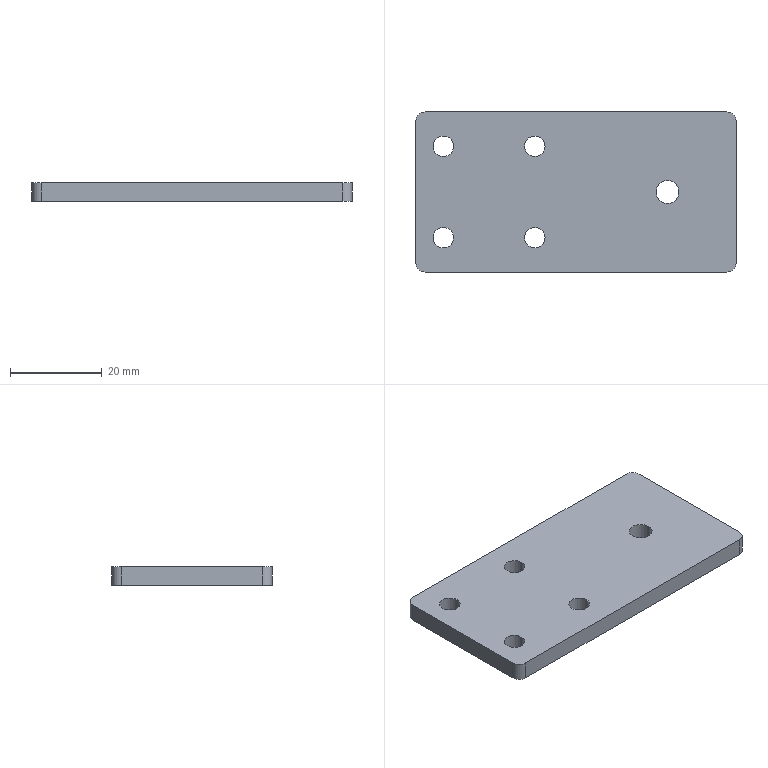Part | NX | features BREP 1 | 1 solid | 20 faces | box 70 x 35 x 4 mm | volume 9453 mm3 | cylinder 14 | plane 6 | commonest cylinder face diameters 4.5 x8 4 x4 5 x2
STEP:
#1=CARTESIAN_POINT('',(33.,-17.5,4.));
#2=VERTEX_POINT('',#1);
#3=CARTESIAN_POINT('',(35.,-15.5,4.));
#4=VERTEX_POINT('',#3);
#5=CARTESIAN_POINT('',(33.,-15.5,4.));
#6=DIRECTION('',(0.,0.,1.));
#7=DIRECTION('',(1.,0.,0.));
#8=AXIS2_PLACEMENT_3D('',#5,#6,#7);
#9=CIRCLE('',#8,2.);
#10=EDGE_CURVE('',#2,#4,#9,.T.);
#11=ORIENTED_EDGE('',*,*,#10,.F.);
#12=CARTESIAN_POINT('',(33.,-17.5,0.));
#13=VERTEX_POINT('',#12);
#14=CARTESIAN_POINT('',(33.,-17.5,4.));
#15=DIRECTION('',(0.,0.,1.));
#16=VECTOR('',#15,1000.);
#17=LINE('',#14,#16);
#18=EDGE_CURVE('',#13,#2,#17,.T.);
#19=ORIENTED_EDGE('',*,*,#18,.F.);
#20=CARTESIAN_POINT('',(35.,-15.5,0.));
#21=VERTEX_POINT('',#20);
#22=CARTESIAN_POINT('',(33.,-15.5,0.));
#23=DIRECTION('',(0.,0.,-1.));
#24=DIRECTION('',(1.,0.,0.));
#25=AXIS2_PLACEMENT_3D('',#22,#23,#24);
#26=CIRCLE('',#25,2.);
#27=EDGE_CURVE('',#21,#13,#26,.T.);
#28=ORIENTED_EDGE('',*,*,#27,.F.);
#29=CARTESIAN_POINT('',(35.,-15.5,4.));
#30=DIRECTION('',(0.,0.,-1.));
#31=VECTOR('',#30,1000.);
#32=LINE('',#29,#31);
#33=EDGE_CURVE('',#4,#21,#32,.T.);
#34=ORIENTED_EDGE('',*,*,#33,.F.);
#35=EDGE_LOOP('',(#11,#19,#28,#34));
#36=FACE_BOUND('',#35,.T.);
#37=CARTESIAN_POINT('',(33.,-15.5,4.));
#38=DIRECTION('',(0.,0.,-1.));
#39=DIRECTION('',(-1.,0.,0.));
#40=AXIS2_PLACEMENT_3D('',#37,#38,#39);
#41=CYLINDRICAL_SURFACE('',#40,2.);
#42=ADVANCED_FACE('',(#36),#41,.T.);
#43=CARTESIAN_POINT('',(35.,15.5,4.));
#44=VERTEX_POINT('',#43);
#45=CARTESIAN_POINT('',(33.,17.5,4.));
#46=VERTEX_POINT('',#45);
#47=CARTESIAN_POINT('',(33.,15.5,4.));
#48=DIRECTION('',(0.,0.,1.));
#49=DIRECTION('',(1.,0.,0.));
#50=AXIS2_PLACEMENT_3D('',#47,#48,#49);
#51=CIRCLE('',#50,2.);
#52=EDGE_CURVE('',#44,#46,#51,.T.);
#53=ORIENTED_EDGE('',*,*,#52,.F.);
#54=CARTESIAN_POINT('',(35.,15.5,0.));
#55=VERTEX_POINT('',#54);
#56=CARTESIAN_POINT('',(35.,15.5,4.));
#57=DIRECTION('',(0.,0.,1.));
#58=VECTOR('',#57,1000.);
#59=LINE('',#56,#58);
#60=EDGE_CURVE('',#55,#44,#59,.T.);
#61=ORIENTED_EDGE('',*,*,#60,.F.);
#62=CARTESIAN_POINT('',(33.,17.5,0.));
#63=VERTEX_POINT('',#62);
#64=CARTESIAN_POINT('',(33.,15.5,0.));
#65=DIRECTION('',(0.,0.,-1.));
#66=DIRECTION('',(1.,0.,0.));
#67=AXIS2_PLACEMENT_3D('',#64,#65,#66);
#68=CIRCLE('',#67,2.);
#69=EDGE_CURVE('',#63,#55,#68,.T.);
#70=ORIENTED_EDGE('',*,*,#69,.F.);
#71=CARTESIAN_POINT('',(33.,17.5,4.));
#72=DIRECTION('',(0.,0.,-1.));
#73=VECTOR('',#72,1000.);
#74=LINE('',#71,#73);
#75=EDGE_CURVE('',#46,#63,#74,.T.);
#76=ORIENTED_EDGE('',*,*,#75,.F.);
#77=EDGE_LOOP('',(#53,#61,#70,#76));
#78=FACE_BOUND('',#77,.T.);
#79=CARTESIAN_POINT('',(33.,15.5,4.));
#80=DIRECTION('',(0.,0.,-1.));
#81=DIRECTION('',(-1.,0.,0.));
#82=AXIS2_PLACEMENT_3D('',#79,#80,#81);
#83=CYLINDRICAL_SURFACE('',#82,2.);
#84=ADVANCED_FACE('',(#78),#83,.T.);
#85=CARTESIAN_POINT('',(-35.,-15.5,4.));
#86=VERTEX_POINT('',#85);
#87=CARTESIAN_POINT('',(-33.,-17.5,4.));
#88=VERTEX_POINT('',#87);
#89=CARTESIAN_POINT('',(-33.,-15.5,4.));
#90=DIRECTION('',(0.,0.,1.));
#91=DIRECTION('',(1.,0.,0.));
#92=AXIS2_PLACEMENT_3D('',#89,#90,#91);
#93=CIRCLE('',#92,2.);
#94=EDGE_CURVE('',#86,#88,#93,.T.);
#95=ORIENTED_EDGE('',*,*,#94,.F.);
#96=CARTESIAN_POINT('',(-35.,-15.5,0.));
#97=VERTEX_POINT('',#96);
#98=CARTESIAN_POINT('',(-35.,-15.5,4.));
#99=DIRECTION('',(0.,0.,1.));
#100=VECTOR('',#99,1000.);
#101=LINE('',#98,#100);
#102=EDGE_CURVE('',#97,#86,#101,.T.);
#103=ORIENTED_EDGE('',*,*,#102,.F.);
#104=CARTESIAN_POINT('',(-33.,-17.5,0.));
#105=VERTEX_POINT('',#104);
#106=CARTESIAN_POINT('',(-33.,-15.5,0.));
#107=DIRECTION('',(0.,0.,-1.));
#108=DIRECTION('',(1.,0.,0.));
#109=AXIS2_PLACEMENT_3D('',#106,#107,#108);
#110=CIRCLE('',#109,2.);
#111=EDGE_CURVE('',#105,#97,#110,.T.);
#112=ORIENTED_EDGE('',*,*,#111,.F.);
#113=CARTESIAN_POINT('',(-33.,-17.5,4.));
#114=DIRECTION('',(0.,0.,-1.));
#115=VECTOR('',#114,1000.);
#116=LINE('',#113,#115);
#117=EDGE_CURVE('',#88,#105,#116,.T.);
#118=ORIENTED_EDGE('',*,*,#117,.F.);
#119=EDGE_LOOP('',(#95,#103,#112,#118));
#120=FACE_BOUND('',#119,.T.);
#121=CARTESIAN_POINT('',(-33.,-15.5,4.));
#122=DIRECTION('',(0.,0.,-1.));
#123=DIRECTION('',(-1.,0.,0.));
#124=AXIS2_PLACEMENT_3D('',#121,#122,#123);
#125=CYLINDRICAL_SURFACE('',#124,2.);
#126=ADVANCED_FACE('',(#120),#125,.T.);
#127=CARTESIAN_POINT('',(-33.,17.5,4.));
#128=VERTEX_POINT('',#127);
#129=CARTESIAN_POINT('',(-35.,15.5,4.));
#130=VERTEX_POINT('',#129);
#131=CARTESIAN_POINT('',(-33.,15.5,4.));
#132=DIRECTION('',(0.,0.,1.));
#133=DIRECTION('',(1.,0.,0.));
#134=AXIS2_PLACEMENT_3D('',#131,#132,#133);
#135=CIRCLE('',#134,2.);
#136=EDGE_CURVE('',#128,#130,#135,.T.);
#137=ORIENTED_EDGE('',*,*,#136,.F.);
#138=CARTESIAN_POINT('',(-33.,17.5,0.));
#139=VERTEX_POINT('',#138);
#140=CARTESIAN_POINT('',(-33.,17.5,4.));
#141=DIRECTION('',(0.,0.,1.));
#142=VECTOR('',#141,1000.);
#143=LINE('',#140,#142);
#144=EDGE_CURVE('',#139,#128,#143,.T.);
#145=ORIENTED_EDGE('',*,*,#144,.F.);
#146=CARTESIAN_POINT('',(-35.,15.5,0.));
#147=VERTEX_POINT('',#146);
#148=CARTESIAN_POINT('',(-33.,15.5,0.));
#149=DIRECTION('',(0.,0.,-1.));
#150=DIRECTION('',(1.,0.,0.));
#151=AXIS2_PLACEMENT_3D('',#148,#149,#150);
#152=CIRCLE('',#151,2.);
#153=EDGE_CURVE('',#147,#139,#152,.T.);
#154=ORIENTED_EDGE('',*,*,#153,.F.);
#155=CARTESIAN_POINT('',(-35.,15.5,4.));
#156=DIRECTION('',(0.,0.,-1.));
#157=VECTOR('',#156,1000.);
#158=LINE('',#155,#157);
#159=EDGE_CURVE('',#130,#147,#158,.T.);
#160=ORIENTED_EDGE('',*,*,#159,.F.);
#161=EDGE_LOOP('',(#137,#145,#154,#160));
#162=FACE_BOUND('',#161,.T.);
#163=CARTESIAN_POINT('',(-33.,15.5,4.));
#164=DIRECTION('',(0.,0.,-1.));
#165=DIRECTION('',(-1.,0.,0.));
#166=AXIS2_PLACEMENT_3D('',#163,#164,#165);
#167=CYLINDRICAL_SURFACE('',#166,2.);
#168=ADVANCED_FACE('',(#162),#167,.T.);
#169=CARTESIAN_POINT('',(-6.75,10.,4.));
#170=VERTEX_POINT('',#169);
#171=CARTESIAN_POINT('',(-6.75,10.,0.));
#172=VERTEX_POINT('',#171);
#173=CARTESIAN_POINT('',(-6.75,10.,0.));
#174=DIRECTION('',(0.,0.,-1.));
#175=VECTOR('',#174,1000.);
#176=LINE('',#173,#175);
#177=EDGE_CURVE('',#170,#172,#176,.T.);
#178=ORIENTED_EDGE('',*,*,#177,.F.);
#179=CARTESIAN_POINT('',(-11.25,10.,4.));
#180=VERTEX_POINT('',#179);
#181=CARTESIAN_POINT('',(-9.,10.,4.));
#182=DIRECTION('',(0.,0.,1.));
#183=DIRECTION('',(1.,0.,0.));
#184=AXIS2_PLACEMENT_3D('',#181,#182,#183);
#185=CIRCLE('',#184,2.25);
#186=EDGE_CURVE('',#170,#180,#185,.T.);
#187=ORIENTED_EDGE('',*,*,#186,.T.);
#188=CARTESIAN_POINT('',(-11.25,10.,0.));
#189=VERTEX_POINT('',#188);
#190=CARTESIAN_POINT('',(-11.25,10.,0.));
#191=DIRECTION('',(0.,0.,-1.));
#192=VECTOR('',#191,1000.);
#193=LINE('',#190,#192);
#194=EDGE_CURVE('',#180,#189,#193,.T.);
#195=ORIENTED_EDGE('',*,*,#194,.T.);
#196=CARTESIAN_POINT('',(-9.,10.,0.));
#197=DIRECTION('',(0.,0.,-1.));
#198=DIRECTION('',(-1.,0.,0.));
#199=AXIS2_PLACEMENT_3D('',#196,#197,#198);
#200=CIRCLE('',#199,2.25);
#201=EDGE_CURVE('',#189,#172,#200,.T.);
#202=ORIENTED_EDGE('',*,*,#201,.T.);
#203=EDGE_LOOP('',(#178,#187,#195,#202));
#204=FACE_BOUND('',#203,.T.);
#205=CARTESIAN_POINT('',(-9.,10.,0.));
#206=DIRECTION('',(0.,0.,-1.));
#207=DIRECTION('',(-1.,0.,0.));
#208=AXIS2_PLACEMENT_3D('',#205,#206,#207);
#209=CYLINDRICAL_SURFACE('',#208,2.25);
#210=ADVANCED_FACE('',(#204),#209,.F.);
#211=CARTESIAN_POINT('',(-26.75,-10.,4.));
#212=VERTEX_POINT('',#211);
#213=CARTESIAN_POINT('',(-26.75,-10.,0.));
#214=VERTEX_POINT('',#213);
#215=CARTESIAN_POINT('',(-26.75,-10.,0.));
#216=DIRECTION('',(0.,0.,-1.));
#217=VECTOR('',#216,1000.);
#218=LINE('',#215,#217);
#219=EDGE_CURVE('',#212,#214,#218,.T.);
#220=ORIENTED_EDGE('',*,*,#219,.F.);
#221=CARTESIAN_POINT('',(-31.25,-10.,4.));
#222=VERTEX_POINT('',#221);
#223=CARTESIAN_POINT('',(-29.,-10.,4.));
#224=DIRECTION('',(0.,0.,1.));
#225=DIRECTION('',(1.,0.,0.));
#226=AXIS2_PLACEMENT_3D('',#223,#224,#225);
#227=CIRCLE('',#226,2.25);
#228=EDGE_CURVE('',#212,#222,#227,.T.);
#229=ORIENTED_EDGE('',*,*,#228,.T.);
#230=CARTESIAN_POINT('',(-31.25,-10.,0.));
#231=VERTEX_POINT('',#230);
#232=CARTESIAN_POINT('',(-31.25,-10.,0.));
#233=DIRECTION('',(0.,0.,-1.));
#234=VECTOR('',#233,1000.);
#235=LINE('',#232,#234);
#236=EDGE_CURVE('',#222,#231,#235,.T.);
#237=ORIENTED_EDGE('',*,*,#236,.T.);
#238=CARTESIAN_POINT('',(-29.,-10.,0.));
#239=DIRECTION('',(0.,0.,-1.));
#240=DIRECTION('',(-1.,0.,0.));
#241=AXIS2_PLACEMENT_3D('',#238,#239,#240);
#242=CIRCLE('',#241,2.25);
#243=EDGE_CURVE('',#231,#214,#242,.T.);
#244=ORIENTED_EDGE('',*,*,#243,.T.);
#245=EDGE_LOOP('',(#220,#229,#237,#244));
#246=FACE_BOUND('',#245,.T.);
#247=CARTESIAN_POINT('',(-29.,-10.,0.));
#248=DIRECTION('',(0.,0.,-1.));
#249=DIRECTION('',(-1.,0.,0.));
#250=AXIS2_PLACEMENT_3D('',#247,#248,#249);
#251=CYLINDRICAL_SURFACE('',#250,2.25);
#252=ADVANCED_FACE('',(#246),#251,.F.);
#253=CARTESIAN_POINT('',(-6.75,-10.,4.));
#254=VERTEX_POINT('',#253);
#255=CARTESIAN_POINT('',(-6.75,-10.,0.));
#256=VERTEX_POINT('',#255);
#257=CARTESIAN_POINT('',(-6.75,-10.,0.));
#258=DIRECTION('',(0.,0.,-1.));
#259=VECTOR('',#258,1000.);
#260=LINE('',#257,#259);
#261=EDGE_CURVE('',#254,#256,#260,.T.);
#262=ORIENTED_EDGE('',*,*,#261,.F.);
#263=CARTESIAN_POINT('',(-11.25,-10.,4.));
#264=VERTEX_POINT('',#263);
#265=CARTESIAN_POINT('',(-9.,-10.,4.));
#266=DIRECTION('',(0.,0.,1.));
#267=DIRECTION('',(1.,0.,0.));
#268=AXIS2_PLACEMENT_3D('',#265,#266,#267);
#269=CIRCLE('',#268,2.25);
#270=EDGE_CURVE('',#254,#264,#269,.T.);
#271=ORIENTED_EDGE('',*,*,#270,.T.);
#272=CARTESIAN_POINT('',(-11.25,-10.,0.));
#273=VERTEX_POINT('',#272);
#274=CARTESIAN_POINT('',(-11.25,-10.,0.));
#275=DIRECTION('',(0.,0.,-1.));
#276=VECTOR('',#275,1000.);
#277=LINE('',#274,#276);
#278=EDGE_CURVE('',#264,#273,#277,.T.);
#279=ORIENTED_EDGE('',*,*,#278,.T.);
#280=CARTESIAN_POINT('',(-9.,-10.,0.));
#281=DIRECTION('',(0.,0.,-1.));
#282=DIRECTION('',(-1.,0.,0.));
#283=AXIS2_PLACEMENT_3D('',#280,#281,#282);
#284=CIRCLE('',#283,2.25);
#285=EDGE_CURVE('',#273,#256,#284,.T.);
#286=ORIENTED_EDGE('',*,*,#285,.T.);
#287=EDGE_LOOP('',(#262,#271,#279,#286));
#288=FACE_BOUND('',#287,.T.);
#289=CARTESIAN_POINT('',(-9.,-10.,0.));
#290=DIRECTION('',(0.,0.,-1.));
#291=DIRECTION('',(-1.,0.,0.));
#292=AXIS2_PLACEMENT_3D('',#289,#290,#291);
#293=CYLINDRICAL_SURFACE('',#292,2.25);
#294=ADVANCED_FACE('',(#288),#293,.F.);
#295=CARTESIAN_POINT('',(-26.75,10.,4.));
#296=VERTEX_POINT('',#295);
#297=CARTESIAN_POINT('',(-26.75,10.,0.));
#298=VERTEX_POINT('',#297);
#299=CARTESIAN_POINT('',(-26.75,10.,0.));
#300=DIRECTION('',(0.,0.,-1.));
#301=VECTOR('',#300,1000.);
#302=LINE('',#299,#301);
#303=EDGE_CURVE('',#296,#298,#302,.T.);
#304=ORIENTED_EDGE('',*,*,#303,.F.);
#305=CARTESIAN_POINT('',(-31.25,10.,4.));
#306=VERTEX_POINT('',#305);
#307=CARTESIAN_POINT('',(-29.,10.,4.));
#308=DIRECTION('',(0.,0.,1.));
#309=DIRECTION('',(1.,0.,0.));
#310=AXIS2_PLACEMENT_3D('',#307,#308,#309);
#311=CIRCLE('',#310,2.25);
#312=EDGE_CURVE('',#296,#306,#311,.T.);
#313=ORIENTED_EDGE('',*,*,#312,.T.);
#314=CARTESIAN_POINT('',(-31.25,10.,0.));
#315=VERTEX_POINT('',#314);
#316=CARTESIAN_POINT('',(-31.25,10.,0.));
#317=DIRECTION('',(0.,0.,-1.));
#318=VECTOR('',#317,1000.);
#319=LINE('',#316,#318);
#320=EDGE_CURVE('',#306,#315,#319,.T.);
#321=ORIENTED_EDGE('',*,*,#320,.T.);
#322=CARTESIAN_POINT('',(-29.,10.,0.));
#323=DIRECTION('',(0.,0.,-1.));
#324=DIRECTION('',(-1.,0.,0.));
#325=AXIS2_PLACEMENT_3D('',#322,#323,#324);
#326=CIRCLE('',#325,2.25);
#327=EDGE_CURVE('',#315,#298,#326,.T.);
#328=ORIENTED_EDGE('',*,*,#327,.T.);
#329=EDGE_LOOP('',(#304,#313,#321,#328));
#330=FACE_BOUND('',#329,.T.);
#331=CARTESIAN_POINT('',(-29.,10.,0.));
#332=DIRECTION('',(0.,0.,-1.));
#333=DIRECTION('',(-1.,0.,0.));
#334=AXIS2_PLACEMENT_3D('',#331,#332,#333);
#335=CYLINDRICAL_SURFACE('',#334,2.25);
#336=ADVANCED_FACE('',(#330),#335,.F.);
#337=CARTESIAN_POINT('',(17.5,0.,4.));
#338=VERTEX_POINT('',#337);
#339=CARTESIAN_POINT('',(17.5,0.,0.));
#340=VERTEX_POINT('',#339);
#341=CARTESIAN_POINT('',(17.5,0.,4.));
#342=DIRECTION('',(0.,0.,1.));
#343=VECTOR('',#342,1000.);
#344=LINE('',#341,#343);
#345=EDGE_CURVE('',#338,#340,#344,.F.);
#346=ORIENTED_EDGE('',*,*,#345,.T.);
#347=CARTESIAN_POINT('',(22.5,0.,0.));
#348=VERTEX_POINT('',#347);
#349=CARTESIAN_POINT('',(20.,0.,0.));
#350=DIRECTION('',(0.,0.,1.));
#351=DIRECTION('',(1.,0.,0.));
#352=AXIS2_PLACEMENT_3D('',#349,#350,#351);
#353=CIRCLE('',#352,2.5);
#354=EDGE_CURVE('',#348,#340,#353,.T.);
#355=ORIENTED_EDGE('',*,*,#354,.F.);
#356=CARTESIAN_POINT('',(22.5,0.,4.));
#357=VERTEX_POINT('',#356);
#358=CARTESIAN_POINT('',(22.5,0.,4.));
#359=DIRECTION('',(0.,0.,1.));
#360=VECTOR('',#359,1000.);
#361=LINE('',#358,#360);
#362=EDGE_CURVE('',#357,#348,#361,.F.);
#363=ORIENTED_EDGE('',*,*,#362,.F.);
#364=CARTESIAN_POINT('',(20.,0.,4.));
#365=DIRECTION('',(0.,0.,1.));
#366=DIRECTION('',(1.,0.,0.));
#367=AXIS2_PLACEMENT_3D('',#364,#365,#366);
#368=CIRCLE('',#367,2.5);
#369=EDGE_CURVE('',#357,#338,#368,.T.);
#370=ORIENTED_EDGE('',*,*,#369,.T.);
#371=EDGE_LOOP('',(#346,#355,#363,#370));
#372=FACE_BOUND('',#371,.T.);
#373=CARTESIAN_POINT('',(20.,0.,4.));
#374=DIRECTION('',(0.,0.,1.));
#375=DIRECTION('',(1.,0.,0.));
#376=AXIS2_PLACEMENT_3D('',#373,#374,#375);
#377=CYLINDRICAL_SURFACE('',#376,2.5);
#378=ADVANCED_FACE('',(#372),#377,.F.);
#379=CARTESIAN_POINT('',(-35.,17.5,0.));
#380=DIRECTION('',(0.,-1.,0.));
#381=VECTOR('',#380,1000.);
#382=LINE('',#379,#381);
#383=EDGE_CURVE('',#147,#97,#382,.T.);
#384=ORIENTED_EDGE('',*,*,#383,.F.);
#385=ORIENTED_EDGE('',*,*,#153,.T.);
#386=CARTESIAN_POINT('',(-35.,17.5,0.));
#387=DIRECTION('',(-1.,0.,0.));
#388=VECTOR('',#387,1000.);
#389=LINE('',#386,#388);
#390=EDGE_CURVE('',#63,#139,#389,.T.);
#391=ORIENTED_EDGE('',*,*,#390,.F.);
#392=ORIENTED_EDGE('',*,*,#69,.T.);
#393=CARTESIAN_POINT('',(35.,17.5,0.));
#394=DIRECTION('',(0.,1.,0.));
#395=VECTOR('',#394,1000.);
#396=LINE('',#393,#395);
#397=EDGE_CURVE('',#21,#55,#396,.T.);
#398=ORIENTED_EDGE('',*,*,#397,.F.);
#399=ORIENTED_EDGE('',*,*,#27,.T.);
#400=CARTESIAN_POINT('',(-35.,-17.5,0.));
#401=DIRECTION('',(1.,0.,0.));
#402=VECTOR('',#401,1000.);
#403=LINE('',#400,#402);
#404=EDGE_CURVE('',#105,#13,#403,.T.);
#405=ORIENTED_EDGE('',*,*,#404,.F.);
#406=ORIENTED_EDGE('',*,*,#111,.T.);
#407=EDGE_LOOP('',(#384,#385,#391,#392,#398,#399,#405,#406));
#408=FACE_BOUND('',#407,.T.);
#409=ORIENTED_EDGE('',*,*,#354,.T.);
#410=CARTESIAN_POINT('',(20.,0.,0.));
#411=DIRECTION('',(0.,0.,1.));
#412=DIRECTION('',(1.,0.,0.));
#413=AXIS2_PLACEMENT_3D('',#410,#411,#412);
#414=CIRCLE('',#413,2.5);
#415=EDGE_CURVE('',#340,#348,#414,.T.);
#416=ORIENTED_EDGE('',*,*,#415,.T.);
#417=EDGE_LOOP('',(#409,#416));
#418=FACE_BOUND('',#417,.T.);
#419=ORIENTED_EDGE('',*,*,#327,.F.);
#420=CARTESIAN_POINT('',(-29.,10.,0.));
#421=DIRECTION('',(0.,0.,-1.));
#422=DIRECTION('',(-1.,0.,0.));
#423=AXIS2_PLACEMENT_3D('',#420,#421,#422);
#424=CIRCLE('',#423,2.25);
#425=EDGE_CURVE('',#298,#315,#424,.T.);
#426=ORIENTED_EDGE('',*,*,#425,.F.);
#427=EDGE_LOOP('',(#419,#426));
#428=FACE_BOUND('',#427,.T.);
#429=ORIENTED_EDGE('',*,*,#285,.F.);
#430=CARTESIAN_POINT('',(-9.,-10.,0.));
#431=DIRECTION('',(0.,0.,-1.));
#432=DIRECTION('',(-1.,0.,0.));
#433=AXIS2_PLACEMENT_3D('',#430,#431,#432);
#434=CIRCLE('',#433,2.25);
#435=EDGE_CURVE('',#256,#273,#434,.T.);
#436=ORIENTED_EDGE('',*,*,#435,.F.);
#437=EDGE_LOOP('',(#429,#436));
#438=FACE_BOUND('',#437,.T.);
#439=ORIENTED_EDGE('',*,*,#243,.F.);
#440=CARTESIAN_POINT('',(-29.,-10.,0.));
#441=DIRECTION('',(0.,0.,-1.));
#442=DIRECTION('',(-1.,0.,0.));
#443=AXIS2_PLACEMENT_3D('',#440,#441,#442);
#444=CIRCLE('',#443,2.25);
#445=EDGE_CURVE('',#214,#231,#444,.T.);
#446=ORIENTED_EDGE('',*,*,#445,.F.);
#447=EDGE_LOOP('',(#439,#446));
#448=FACE_BOUND('',#447,.T.);
#449=ORIENTED_EDGE('',*,*,#201,.F.);
#450=CARTESIAN_POINT('',(-9.,10.,0.));
#451=DIRECTION('',(0.,0.,-1.));
#452=DIRECTION('',(-1.,0.,0.));
#453=AXIS2_PLACEMENT_3D('',#450,#451,#452);
#454=CIRCLE('',#453,2.25);
#455=EDGE_CURVE('',#172,#189,#454,.T.);
#456=ORIENTED_EDGE('',*,*,#455,.F.);
#457=EDGE_LOOP('',(#449,#456));
#458=FACE_BOUND('',#457,.T.);
#459=CARTESIAN_POINT('',(0.,0.,0.));
#460=DIRECTION('',(0.,0.,1.));
#461=DIRECTION('',(1.,0.,0.));
#462=AXIS2_PLACEMENT_3D('',#459,#460,#461);
#463=PLANE('',#462);
#464=ADVANCED_FACE('',(#408,#418,#428,#438,#448,#458),#463,.F.);
#465=CARTESIAN_POINT('',(-35.,17.5,4.));
#466=DIRECTION('',(-1.,0.,0.));
#467=VECTOR('',#466,1000.);
#468=LINE('',#465,#467);
#469=EDGE_CURVE('',#46,#128,#468,.T.);
#470=ORIENTED_EDGE('',*,*,#469,.T.);
#471=ORIENTED_EDGE('',*,*,#136,.T.);
#472=CARTESIAN_POINT('',(-35.,17.5,4.));
#473=DIRECTION('',(0.,-1.,0.));
#474=VECTOR('',#473,1000.);
#475=LINE('',#472,#474);
#476=EDGE_CURVE('',#130,#86,#475,.T.);
#477=ORIENTED_EDGE('',*,*,#476,.T.);
#478=ORIENTED_EDGE('',*,*,#94,.T.);
#479=CARTESIAN_POINT('',(-35.,-17.5,4.));
#480=DIRECTION('',(1.,0.,0.));
#481=VECTOR('',#480,1000.);
#482=LINE('',#479,#481);
#483=EDGE_CURVE('',#88,#2,#482,.T.);
#484=ORIENTED_EDGE('',*,*,#483,.T.);
#485=ORIENTED_EDGE('',*,*,#10,.T.);
#486=CARTESIAN_POINT('',(35.,17.5,4.));
#487=DIRECTION('',(0.,1.,0.));
#488=VECTOR('',#487,1000.);
#489=LINE('',#486,#488);
#490=EDGE_CURVE('',#4,#44,#489,.T.);
#491=ORIENTED_EDGE('',*,*,#490,.T.);
#492=ORIENTED_EDGE('',*,*,#52,.T.);
#493=EDGE_LOOP('',(#470,#471,#477,#478,#484,#485,#491,#492));
#494=FACE_BOUND('',#493,.T.);
#495=ORIENTED_EDGE('',*,*,#369,.F.);
#496=CARTESIAN_POINT('',(20.,0.,4.));
#497=DIRECTION('',(0.,0.,1.));
#498=DIRECTION('',(1.,0.,0.));
#499=AXIS2_PLACEMENT_3D('',#496,#497,#498);
#500=CIRCLE('',#499,2.5);
#501=EDGE_CURVE('',#338,#357,#500,.T.);
#502=ORIENTED_EDGE('',*,*,#501,.F.);
#503=EDGE_LOOP('',(#495,#502));
#504=FACE_BOUND('',#503,.T.);
#505=CARTESIAN_POINT('',(-29.,10.,4.));
#506=DIRECTION('',(0.,0.,1.));
#507=DIRECTION('',(1.,0.,0.));
#508=AXIS2_PLACEMENT_3D('',#505,#506,#507);
#509=CIRCLE('',#508,2.25);
#510=EDGE_CURVE('',#306,#296,#509,.T.);
#511=ORIENTED_EDGE('',*,*,#510,.F.);
#512=ORIENTED_EDGE('',*,*,#312,.F.);
#513=EDGE_LOOP('',(#511,#512));
#514=FACE_BOUND('',#513,.T.);
#515=CARTESIAN_POINT('',(-9.,-10.,4.));
#516=DIRECTION('',(0.,0.,1.));
#517=DIRECTION('',(1.,0.,0.));
#518=AXIS2_PLACEMENT_3D('',#515,#516,#517);
#519=CIRCLE('',#518,2.25);
#520=EDGE_CURVE('',#264,#254,#519,.T.);
#521=ORIENTED_EDGE('',*,*,#520,.F.);
#522=ORIENTED_EDGE('',*,*,#270,.F.);
#523=EDGE_LOOP('',(#521,#522));
#524=FACE_BOUND('',#523,.T.);
#525=CARTESIAN_POINT('',(-29.,-10.,4.));
#526=DIRECTION('',(0.,0.,1.));
#527=DIRECTION('',(1.,0.,0.));
#528=AXIS2_PLACEMENT_3D('',#525,#526,#527);
#529=CIRCLE('',#528,2.25);
#530=EDGE_CURVE('',#222,#212,#529,.T.);
#531=ORIENTED_EDGE('',*,*,#530,.F.);
#532=ORIENTED_EDGE('',*,*,#228,.F.);
#533=EDGE_LOOP('',(#531,#532));
#534=FACE_BOUND('',#533,.T.);
#535=CARTESIAN_POINT('',(-9.,10.,4.));
#536=DIRECTION('',(0.,0.,1.));
#537=DIRECTION('',(1.,0.,0.));
#538=AXIS2_PLACEMENT_3D('',#535,#536,#537);
#539=CIRCLE('',#538,2.25);
#540=EDGE_CURVE('',#180,#170,#539,.T.);
#541=ORIENTED_EDGE('',*,*,#540,.F.);
#542=ORIENTED_EDGE('',*,*,#186,.F.);
#543=EDGE_LOOP('',(#541,#542));
#544=FACE_BOUND('',#543,.T.);
#545=CARTESIAN_POINT('',(0.,0.,4.));
#546=DIRECTION('',(0.,0.,1.));
#547=DIRECTION('',(1.,0.,0.));
#548=AXIS2_PLACEMENT_3D('',#545,#546,#547);
#549=PLANE('',#548);
#550=ADVANCED_FACE('',(#494,#504,#514,#524,#534,#544),#549,.T.);
#551=ORIENTED_EDGE('',*,*,#483,.F.);
#552=ORIENTED_EDGE('',*,*,#117,.T.);
#553=ORIENTED_EDGE('',*,*,#404,.T.);
#554=ORIENTED_EDGE('',*,*,#18,.T.);
#555=EDGE_LOOP('',(#551,#552,#553,#554));
#556=FACE_BOUND('',#555,.T.);
#557=CARTESIAN_POINT('',(-35.,-17.5,4.));
#558=DIRECTION('',(0.,1.,0.));
#559=DIRECTION('',(0.,0.,1.));
#560=AXIS2_PLACEMENT_3D('',#557,#558,#559);
#561=PLANE('',#560);
#562=ADVANCED_FACE('',(#556),#561,.F.);
#563=ORIENTED_EDGE('',*,*,#476,.F.);
#564=ORIENTED_EDGE('',*,*,#159,.T.);
#565=ORIENTED_EDGE('',*,*,#383,.T.);
#566=ORIENTED_EDGE('',*,*,#102,.T.);
#567=EDGE_LOOP('',(#563,#564,#565,#566));
#568=FACE_BOUND('',#567,.T.);
#569=CARTESIAN_POINT('',(-35.,17.5,4.));
#570=DIRECTION('',(1.,0.,0.));
#571=DIRECTION('',(0.,0.,-1.));
#572=AXIS2_PLACEMENT_3D('',#569,#570,#571);
#573=PLANE('',#572);
#574=ADVANCED_FACE('',(#568),#573,.F.);
#575=ORIENTED_EDGE('',*,*,#390,.T.);
#576=ORIENTED_EDGE('',*,*,#144,.T.);
#577=ORIENTED_EDGE('',*,*,#469,.F.);
#578=ORIENTED_EDGE('',*,*,#75,.T.);
#579=EDGE_LOOP('',(#575,#576,#577,#578));
#580=FACE_BOUND('',#579,.T.);
#581=CARTESIAN_POINT('',(-35.,17.5,4.));
#582=DIRECTION('',(0.,-1.,0.));
#583=DIRECTION('',(0.,0.,-1.));
#584=AXIS2_PLACEMENT_3D('',#581,#582,#583);
#585=PLANE('',#584);
#586=ADVANCED_FACE('',(#580),#585,.F.);
#587=ORIENTED_EDGE('',*,*,#397,.T.);
#588=ORIENTED_EDGE('',*,*,#60,.T.);
#589=ORIENTED_EDGE('',*,*,#490,.F.);
#590=ORIENTED_EDGE('',*,*,#33,.T.);
#591=EDGE_LOOP('',(#587,#588,#589,#590));
#592=FACE_BOUND('',#591,.T.);
#593=CARTESIAN_POINT('',(35.,17.5,4.));
#594=DIRECTION('',(-1.,0.,0.));
#595=DIRECTION('',(0.,-1.,0.));
#596=AXIS2_PLACEMENT_3D('',#593,#594,#595);
#597=PLANE('',#596);
#598=ADVANCED_FACE('',(#592),#597,.F.);
#599=ORIENTED_EDGE('',*,*,#415,.F.);
#600=ORIENTED_EDGE('',*,*,#345,.F.);
#601=ORIENTED_EDGE('',*,*,#501,.T.);
#602=ORIENTED_EDGE('',*,*,#362,.T.);
#603=EDGE_LOOP('',(#599,#600,#601,#602));
#604=FACE_BOUND('',#603,.T.);
#605=CARTESIAN_POINT('',(20.,0.,4.));
#606=DIRECTION('',(0.,0.,1.));
#607=DIRECTION('',(1.,0.,0.));
#608=AXIS2_PLACEMENT_3D('',#605,#606,#607);
#609=CYLINDRICAL_SURFACE('',#608,2.5);
#610=ADVANCED_FACE('',(#604),#609,.F.);
#611=ORIENTED_EDGE('',*,*,#510,.T.);
#612=ORIENTED_EDGE('',*,*,#303,.T.);
#613=ORIENTED_EDGE('',*,*,#425,.T.);
#614=ORIENTED_EDGE('',*,*,#320,.F.);
#615=EDGE_LOOP('',(#611,#612,#613,#614));
#616=FACE_BOUND('',#615,.T.);
#617=CARTESIAN_POINT('',(-29.,10.,0.));
#618=DIRECTION('',(0.,0.,-1.));
#619=DIRECTION('',(-1.,0.,0.));
#620=AXIS2_PLACEMENT_3D('',#617,#618,#619);
#621=CYLINDRICAL_SURFACE('',#620,2.25);
#622=ADVANCED_FACE('',(#616),#621,.F.);
#623=ORIENTED_EDGE('',*,*,#520,.T.);
#624=ORIENTED_EDGE('',*,*,#261,.T.);
#625=ORIENTED_EDGE('',*,*,#435,.T.);
#626=ORIENTED_EDGE('',*,*,#278,.F.);
#627=EDGE_LOOP('',(#623,#624,#625,#626));
#628=FACE_BOUND('',#627,.T.);
#629=CARTESIAN_POINT('',(-9.,-10.,0.));
#630=DIRECTION('',(0.,0.,-1.));
#631=DIRECTION('',(-1.,0.,0.));
#632=AXIS2_PLACEMENT_3D('',#629,#630,#631);
#633=CYLINDRICAL_SURFACE('',#632,2.25);
#634=ADVANCED_FACE('',(#628),#633,.F.);
#635=ORIENTED_EDGE('',*,*,#530,.T.);
#636=ORIENTED_EDGE('',*,*,#219,.T.);
#637=ORIENTED_EDGE('',*,*,#445,.T.);
#638=ORIENTED_EDGE('',*,*,#236,.F.);
#639=EDGE_LOOP('',(#635,#636,#637,#638));
#640=FACE_BOUND('',#639,.T.);
#641=CARTESIAN_POINT('',(-29.,-10.,0.));
#642=DIRECTION('',(0.,0.,-1.));
#643=DIRECTION('',(-1.,0.,0.));
#644=AXIS2_PLACEMENT_3D('',#641,#642,#643);
#645=CYLINDRICAL_SURFACE('',#644,2.25);
#646=ADVANCED_FACE('',(#640),#645,.F.);
#647=ORIENTED_EDGE('',*,*,#540,.T.);
#648=ORIENTED_EDGE('',*,*,#177,.T.);
#649=ORIENTED_EDGE('',*,*,#455,.T.);
#650=ORIENTED_EDGE('',*,*,#194,.F.);
#651=EDGE_LOOP('',(#647,#648,#649,#650));
#652=FACE_BOUND('',#651,.T.);
#653=CARTESIAN_POINT('',(-9.,10.,0.));
#654=DIRECTION('',(0.,0.,-1.));
#655=DIRECTION('',(-1.,0.,0.));
#656=AXIS2_PLACEMENT_3D('',#653,#654,#655);
#657=CYLINDRICAL_SURFACE('',#656,2.25);
#658=ADVANCED_FACE('',(#652),#657,.F.);
#659=CLOSED_SHELL('',(#42,#84,#126,#168,#210,#252,#294,#336,#378,#464,#550,#562,#574,#586,#598,#610,#622,#634,#646,#658));
#660=MANIFOLD_SOLID_BREP('',#659);
#661=(LENGTH_UNIT()NAMED_UNIT(*)SI_UNIT(.MILLI.,.METRE.));
#662=UNCERTAINTY_MEASURE_WITH_UNIT(LENGTH_MEASURE(0.00001),#661,'','');
#663=(NAMED_UNIT(*)PLANE_ANGLE_UNIT()SI_UNIT($,.RADIAN.));
#664=(NAMED_UNIT(*)SI_UNIT($,.STERADIAN.)SOLID_ANGLE_UNIT());
#665=(GEOMETRIC_REPRESENTATION_CONTEXT(3)GLOBAL_UNCERTAINTY_ASSIGNED_CONTEXT((#662))GLOBAL_UNIT_ASSIGNED_CONTEXT((#661,#663,#664))REPRESENTATION_CONTEXT('',''));
#666=ADVANCED_BREP_SHAPE_REPRESENTATION('',(#660),#665);